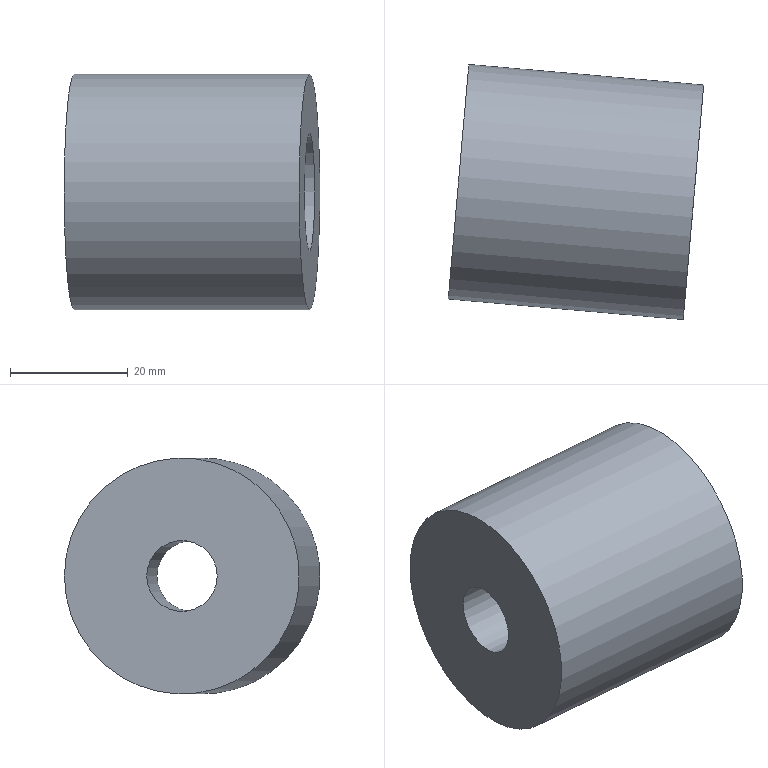Part | NX | features solid 2 | 1 solid | 6 faces | box 43.334 x 43.334 x 40 mm | volume 41720 mm3 | cylinder 3 | plane 3 | commonest cylinder face diameters 12 x1 20 x1 40 x1
STEP:
#1=CARTESIAN_POINT('',(-533.465,327.742,-245.));
#2=VERTEX_POINT('',#1);
#3=CARTESIAN_POINT('',(-535.209,307.818,-245.));
#4=DIRECTION('',(0.9962,-0.08716,0.));
#5=DIRECTION('',(0.08716,0.9962,0.));
#6=AXIS2_PLACEMENT_3D('',#3,#4,#5);
#7=CIRCLE('',#6,20.);
#8=EDGE_CURVE('',#2,#2,#7,.T.);
#9=ORIENTED_EDGE('',*,*,#8,.T.);
#10=EDGE_LOOP('',(#9));
#11=FACE_BOUND('',#10,.T.);
#12=CARTESIAN_POINT('',(-493.618,324.256,-245.));
#13=VERTEX_POINT('',#12);
#14=CARTESIAN_POINT('',(-495.361,304.332,-245.));
#15=DIRECTION('',(0.9962,-0.08716,0.));
#16=DIRECTION('',(0.08716,0.9962,0.));
#17=AXIS2_PLACEMENT_3D('',#14,#15,#16);
#18=CIRCLE('',#17,20.);
#19=EDGE_CURVE('',#13,#13,#18,.T.);
#20=ORIENTED_EDGE('',*,*,#19,.F.);
#21=EDGE_LOOP('',(#20));
#22=FACE_BOUND('',#21,.T.);
#23=CARTESIAN_POINT('',(-535.209,307.818,-245.));
#24=DIRECTION('',(0.9962,-0.08716,0.));
#25=DIRECTION('',(-0.08716,-0.9962,0.));
#26=AXIS2_PLACEMENT_3D('',#23,#24,#25);
#27=CYLINDRICAL_SURFACE('',#26,20.);
#28=ADVANCED_FACE('',(#11,#22),#27,.T.);
#29=CARTESIAN_POINT('',(-534.686,313.795,-245.));
#30=VERTEX_POINT('',#29);
#31=CARTESIAN_POINT('',(-535.209,307.818,-245.));
#32=DIRECTION('',(0.9962,-0.08716,0.));
#33=DIRECTION('',(0.08716,0.9962,0.));
#34=AXIS2_PLACEMENT_3D('',#31,#32,#33);
#35=CIRCLE('',#34,6.);
#36=EDGE_CURVE('',#30,#30,#35,.T.);
#37=ORIENTED_EDGE('',*,*,#36,.T.);
#38=EDGE_LOOP('',(#37));
#39=FACE_BOUND('',#38,.T.);
#40=ORIENTED_EDGE('',*,*,#8,.F.);
#41=EDGE_LOOP('',(#40));
#42=FACE_BOUND('',#41,.T.);
#43=CARTESIAN_POINT('',(-535.209,307.818,-245.));
#44=DIRECTION('',(-0.9962,0.08716,0.));
#45=DIRECTION('',(0.08716,0.9962,0.));
#46=AXIS2_PLACEMENT_3D('',#43,#44,#45);
#47=PLANE('',#46);
#48=ADVANCED_FACE('',(#39,#42),#47,.T.);
#49=CARTESIAN_POINT('',(-494.489,314.294,-245.));
#50=VERTEX_POINT('',#49);
#51=CARTESIAN_POINT('',(-495.361,304.332,-245.));
#52=DIRECTION('',(0.9962,-0.08716,0.));
#53=DIRECTION('',(0.08716,0.9962,0.));
#54=AXIS2_PLACEMENT_3D('',#51,#52,#53);
#55=CIRCLE('',#54,10.);
#56=EDGE_CURVE('',#50,#50,#55,.T.);
#57=ORIENTED_EDGE('',*,*,#56,.F.);
#58=EDGE_LOOP('',(#57));
#59=FACE_BOUND('',#58,.T.);
#60=ORIENTED_EDGE('',*,*,#19,.T.);
#61=EDGE_LOOP('',(#60));
#62=FACE_BOUND('',#61,.T.);
#63=CARTESIAN_POINT('',(-495.361,304.332,-245.));
#64=DIRECTION('',(-0.9962,0.08716,0.));
#65=DIRECTION('',(0.08716,0.9962,0.));
#66=AXIS2_PLACEMENT_3D('',#63,#64,#65);
#67=PLANE('',#66);
#68=ADVANCED_FACE('',(#59,#62),#67,.F.);
#69=CARTESIAN_POINT('',(-514.762,312.052,-245.));
#70=VERTEX_POINT('',#69);
#71=CARTESIAN_POINT('',(-515.285,306.075,-245.));
#72=DIRECTION('',(0.9962,-0.08716,0.));
#73=DIRECTION('',(0.08716,0.9962,0.));
#74=AXIS2_PLACEMENT_3D('',#71,#72,#73);
#75=CIRCLE('',#74,6.);
#76=EDGE_CURVE('',#70,#70,#75,.T.);
#77=ORIENTED_EDGE('',*,*,#76,.F.);
#78=EDGE_LOOP('',(#77));
#79=FACE_BOUND('',#78,.T.);
#80=CARTESIAN_POINT('',(-514.413,316.037,-245.));
#81=VERTEX_POINT('',#80);
#82=CARTESIAN_POINT('',(-515.285,306.075,-245.));
#83=DIRECTION('',(0.9962,-0.08716,0.));
#84=DIRECTION('',(0.08716,0.9962,0.));
#85=AXIS2_PLACEMENT_3D('',#82,#83,#84);
#86=CIRCLE('',#85,10.);
#87=EDGE_CURVE('',#81,#81,#86,.T.);
#88=ORIENTED_EDGE('',*,*,#87,.T.);
#89=EDGE_LOOP('',(#88));
#90=FACE_BOUND('',#89,.T.);
#91=CARTESIAN_POINT('',(-515.285,306.075,-245.));
#92=DIRECTION('',(-0.9962,0.08716,0.));
#93=DIRECTION('',(0.08716,0.9962,0.));
#94=AXIS2_PLACEMENT_3D('',#91,#92,#93);
#95=PLANE('',#94);
#96=ADVANCED_FACE('',(#79,#90),#95,.F.);
#97=ORIENTED_EDGE('',*,*,#87,.F.);
#98=EDGE_LOOP('',(#97));
#99=FACE_BOUND('',#98,.T.);
#100=ORIENTED_EDGE('',*,*,#56,.T.);
#101=EDGE_LOOP('',(#100));
#102=FACE_BOUND('',#101,.T.);
#103=CARTESIAN_POINT('',(-495.361,304.332,-245.));
#104=DIRECTION('',(-0.9962,0.08716,0.));
#105=DIRECTION('',(0.08716,0.9962,0.));
#106=AXIS2_PLACEMENT_3D('',#103,#104,#105);
#107=CYLINDRICAL_SURFACE('',#106,10.);
#108=ADVANCED_FACE('',(#99,#102),#107,.F.);
#109=ORIENTED_EDGE('',*,*,#36,.F.);
#110=EDGE_LOOP('',(#109));
#111=FACE_BOUND('',#110,.T.);
#112=ORIENTED_EDGE('',*,*,#76,.T.);
#113=EDGE_LOOP('',(#112));
#114=FACE_BOUND('',#113,.T.);
#115=CARTESIAN_POINT('',(-515.285,306.075,-245.));
#116=DIRECTION('',(-0.9962,0.08716,0.));
#117=DIRECTION('',(0.08716,0.9962,0.));
#118=AXIS2_PLACEMENT_3D('',#115,#116,#117);
#119=CYLINDRICAL_SURFACE('',#118,6.);
#120=ADVANCED_FACE('',(#111,#114),#119,.F.);
#121=CLOSED_SHELL('',(#28,#48,#68,#96,#108,#120));
#122=MANIFOLD_SOLID_BREP('',#121);
#123=(LENGTH_UNIT()NAMED_UNIT(*)SI_UNIT(.MILLI.,.METRE.));
#124=UNCERTAINTY_MEASURE_WITH_UNIT(LENGTH_MEASURE(0.00001),#123,'','');
#125=(NAMED_UNIT(*)PLANE_ANGLE_UNIT()SI_UNIT($,.RADIAN.));
#126=(NAMED_UNIT(*)SI_UNIT($,.STERADIAN.)SOLID_ANGLE_UNIT());
#127=(GEOMETRIC_REPRESENTATION_CONTEXT(3)GLOBAL_UNCERTAINTY_ASSIGNED_CONTEXT((#124))GLOBAL_UNIT_ASSIGNED_CONTEXT((#123,#125,#126))REPRESENTATION_CONTEXT('',''));
#128=ADVANCED_BREP_SHAPE_REPRESENTATION('',(#122),#127);